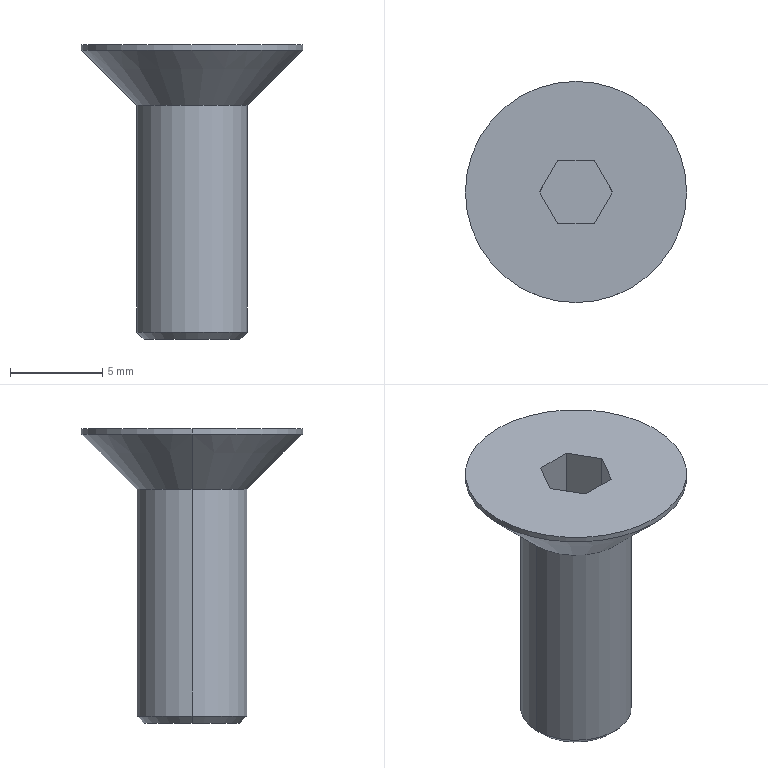Part | Creo | 1 solid | 17 faces | box 12 x 12 x 16 mm | volume 548.89 mm3 | plane 9 | cone 4 | cylinder 4 | commonest cylinder face diameters 6 x2 12 x2
STEP:
#1=CARTESIAN_POINT('',(-332.6,330.,200.));
#2=VERTEX_POINT('',#1);
#3=CARTESIAN_POINT('',(-327.4,330.,200.));
#4=VERTEX_POINT('',#3);
#5=CARTESIAN_POINT('',(-330.,330.,200.));
#6=DIRECTION('',(0.,0.,-1.));
#7=DIRECTION('',(-1.,0.,0.));
#8=AXIS2_PLACEMENT_3D('',#5,#6,#7);
#9=CIRCLE('',#8,2.6);
#10=EDGE_CURVE('',#2,#4,#9,.T.);
#11=ORIENTED_EDGE('',*,*,#10,.F.);
#12=CARTESIAN_POINT('',(-330.,330.,200.));
#13=DIRECTION('',(0.,0.,-1.));
#14=DIRECTION('',(1.,0.,0.));
#15=AXIS2_PLACEMENT_3D('',#12,#13,#14);
#16=CIRCLE('',#15,2.6);
#17=EDGE_CURVE('',#4,#2,#16,.T.);
#18=ORIENTED_EDGE('',*,*,#17,.F.);
#19=EDGE_LOOP('',(#11,#18));
#20=FACE_OUTER_BOUND('',#19,.F.);
#21=CARTESIAN_POINT('',(-326.825,330.,200.));
#22=DIRECTION('',(0.,0.,-1.));
#23=DIRECTION('',(-1.,0.,0.));
#24=AXIS2_PLACEMENT_3D('',#21,#22,#23);
#25=PLANE('',#24);
#26=ADVANCED_FACE('',(#20),#25,.T.);
#27=CARTESIAN_POINT('',(-333.,330.,200.4));
#28=VERTEX_POINT('',#27);
#29=CARTESIAN_POINT('',(-327.,330.,200.4));
#30=VERTEX_POINT('',#29);
#31=CARTESIAN_POINT('',(-330.,330.,200.4));
#32=DIRECTION('',(0.,0.,-1.));
#33=DIRECTION('',(-1.,0.,0.));
#34=AXIS2_PLACEMENT_3D('',#31,#32,#33);
#35=CIRCLE('',#34,3.);
#36=EDGE_CURVE('',#28,#30,#35,.T.);
#37=ORIENTED_EDGE('',*,*,#36,.F.);
#38=CARTESIAN_POINT('',(-332.6,330.,200.));
#39=DIRECTION('',(-0.7071,0.,0.7071));
#40=VECTOR('',#39,0.5657);
#41=LINE('',#38,#40);
#42=EDGE_CURVE('',#2,#28,#41,.T.);
#43=ORIENTED_EDGE('',*,*,#42,.F.);
#44=ORIENTED_EDGE('',*,*,#10,.T.);
#45=CARTESIAN_POINT('',(-327.4,330.,200.));
#46=DIRECTION('',(0.7071,0.,0.7071));
#47=VECTOR('',#46,0.5657);
#48=LINE('',#45,#47);
#49=EDGE_CURVE('',#4,#30,#48,.T.);
#50=ORIENTED_EDGE('',*,*,#49,.T.);
#51=EDGE_LOOP('',(#37,#43,#44,#50));
#52=FACE_OUTER_BOUND('',#51,.F.);
#53=CARTESIAN_POINT('',(-330.,330.,200.2));
#54=DIRECTION('',(0.,0.,1.));
#55=DIRECTION('',(1.,0.,0.));
#56=AXIS2_PLACEMENT_3D('',#53,#54,#55);
#57=CONICAL_SURFACE('',#56,2.8,45.);
#58=ADVANCED_FACE('',(#52),#57,.T.);
#59=ORIENTED_EDGE('',*,*,#36,.T.);
#60=CARTESIAN_POINT('',(-327.,330.,212.7));
#61=VERTEX_POINT('',#60);
#62=CARTESIAN_POINT('',(-327.,330.,200.4));
#63=DIRECTION('',(0.,0.,1.));
#64=VECTOR('',#63,12.3);
#65=LINE('',#62,#64);
#66=EDGE_CURVE('',#30,#61,#65,.T.);
#67=ORIENTED_EDGE('',*,*,#66,.T.);
#68=CARTESIAN_POINT('',(-333.,330.,212.7));
#69=VERTEX_POINT('',#68);
#70=CARTESIAN_POINT('',(-330.,330.,212.7));
#71=DIRECTION('',(0.,0.,1.));
#72=DIRECTION('',(1.,0.,0.));
#73=AXIS2_PLACEMENT_3D('',#70,#71,#72);
#74=CIRCLE('',#73,3.);
#75=EDGE_CURVE('',#61,#69,#74,.T.);
#76=ORIENTED_EDGE('',*,*,#75,.T.);
#77=CARTESIAN_POINT('',(-333.,330.,200.4));
#78=DIRECTION('',(0.,0.,1.));
#79=VECTOR('',#78,12.3);
#80=LINE('',#77,#79);
#81=EDGE_CURVE('',#28,#69,#80,.T.);
#82=ORIENTED_EDGE('',*,*,#81,.F.);
#83=EDGE_LOOP('',(#59,#67,#76,#82));
#84=FACE_OUTER_BOUND('',#83,.F.);
#85=CARTESIAN_POINT('',(-330.,330.,216.307));
#86=DIRECTION('',(0.,0.,1.));
#87=DIRECTION('',(1.,0.,0.));
#88=AXIS2_PLACEMENT_3D('',#85,#86,#87);
#89=CYLINDRICAL_SURFACE('',#88,3.);
#90=ADVANCED_FACE('',(#84),#89,.T.);
#91=CARTESIAN_POINT('',(-330.,330.,200.4));
#92=DIRECTION('',(0.,0.,-1.));
#93=DIRECTION('',(1.,0.,0.));
#94=AXIS2_PLACEMENT_3D('',#91,#92,#93);
#95=CIRCLE('',#94,3.);
#96=EDGE_CURVE('',#30,#28,#95,.T.);
#97=ORIENTED_EDGE('',*,*,#96,.T.);
#98=ORIENTED_EDGE('',*,*,#81,.T.);
#99=CARTESIAN_POINT('',(-330.,330.,212.7));
#100=DIRECTION('',(0.,0.,1.));
#101=DIRECTION('',(-1.,0.,0.));
#102=AXIS2_PLACEMENT_3D('',#99,#100,#101);
#103=CIRCLE('',#102,3.);
#104=EDGE_CURVE('',#69,#61,#103,.T.);
#105=ORIENTED_EDGE('',*,*,#104,.T.);
#106=ORIENTED_EDGE('',*,*,#66,.F.);
#107=EDGE_LOOP('',(#97,#98,#105,#106));
#108=FACE_OUTER_BOUND('',#107,.F.);
#109=CARTESIAN_POINT('',(-330.,330.,216.307));
#110=DIRECTION('',(0.,0.,1.));
#111=DIRECTION('',(1.,0.,0.));
#112=AXIS2_PLACEMENT_3D('',#109,#110,#111);
#113=CYLINDRICAL_SURFACE('',#112,3.);
#114=ADVANCED_FACE('',(#108),#113,.T.);
#115=ORIENTED_EDGE('',*,*,#96,.F.);
#116=ORIENTED_EDGE('',*,*,#49,.F.);
#117=ORIENTED_EDGE('',*,*,#17,.T.);
#118=ORIENTED_EDGE('',*,*,#42,.T.);
#119=EDGE_LOOP('',(#115,#116,#117,#118));
#120=FACE_OUTER_BOUND('',#119,.F.);
#121=CARTESIAN_POINT('',(-330.,330.,200.2));
#122=DIRECTION('',(0.,0.,1.));
#123=DIRECTION('',(1.,0.,0.));
#124=AXIS2_PLACEMENT_3D('',#121,#122,#123);
#125=CONICAL_SURFACE('',#124,2.8,45.);
#126=ADVANCED_FACE('',(#120),#125,.T.);
#127=ORIENTED_EDGE('',*,*,#104,.F.);
#128=CARTESIAN_POINT('',(-336.,330.,215.7));
#129=VERTEX_POINT('',#128);
#130=CARTESIAN_POINT('',(-333.,330.,212.7));
#131=DIRECTION('',(-0.7071,0.,0.7071));
#132=VECTOR('',#131,4.243);
#133=LINE('',#130,#132);
#134=EDGE_CURVE('',#69,#129,#133,.T.);
#135=ORIENTED_EDGE('',*,*,#134,.T.);
#136=CARTESIAN_POINT('',(-324.,330.,215.7));
#137=VERTEX_POINT('',#136);
#138=CARTESIAN_POINT('',(-330.,330.,215.7));
#139=DIRECTION('',(0.,0.,-1.));
#140=DIRECTION('',(1.,0.,0.));
#141=AXIS2_PLACEMENT_3D('',#138,#139,#140);
#142=CIRCLE('',#141,6.);
#143=EDGE_CURVE('',#137,#129,#142,.T.);
#144=ORIENTED_EDGE('',*,*,#143,.F.);
#145=CARTESIAN_POINT('',(-327.,330.,212.7));
#146=DIRECTION('',(0.7071,0.,0.7071));
#147=VECTOR('',#146,4.243);
#148=LINE('',#145,#147);
#149=EDGE_CURVE('',#61,#137,#148,.T.);
#150=ORIENTED_EDGE('',*,*,#149,.F.);
#151=EDGE_LOOP('',(#127,#135,#144,#150));
#152=FACE_OUTER_BOUND('',#151,.F.);
#153=CARTESIAN_POINT('',(-330.,330.,214.2));
#154=DIRECTION('',(0.,0.,1.));
#155=DIRECTION('',(1.,0.,0.));
#156=AXIS2_PLACEMENT_3D('',#153,#154,#155);
#157=CONICAL_SURFACE('',#156,4.5,45.);
#158=ADVANCED_FACE('',(#152),#157,.T.);
#159=ORIENTED_EDGE('',*,*,#75,.F.);
#160=ORIENTED_EDGE('',*,*,#149,.T.);
#161=CARTESIAN_POINT('',(-330.,330.,215.7));
#162=DIRECTION('',(0.,0.,-1.));
#163=DIRECTION('',(-1.,0.,0.));
#164=AXIS2_PLACEMENT_3D('',#161,#162,#163);
#165=CIRCLE('',#164,6.);
#166=EDGE_CURVE('',#129,#137,#165,.T.);
#167=ORIENTED_EDGE('',*,*,#166,.F.);
#168=ORIENTED_EDGE('',*,*,#134,.F.);
#169=EDGE_LOOP('',(#159,#160,#167,#168));
#170=FACE_OUTER_BOUND('',#169,.F.);
#171=CARTESIAN_POINT('',(-330.,330.,214.2));
#172=DIRECTION('',(0.,0.,1.));
#173=DIRECTION('',(1.,0.,0.));
#174=AXIS2_PLACEMENT_3D('',#171,#172,#173);
#175=CONICAL_SURFACE('',#174,4.5,45.);
#176=ADVANCED_FACE('',(#170),#175,.T.);
#177=ORIENTED_EDGE('',*,*,#166,.T.);
#178=CARTESIAN_POINT('',(-324.,330.,216.));
#179=VERTEX_POINT('',#178);
#180=CARTESIAN_POINT('',(-324.,330.,215.7));
#181=DIRECTION('',(0.,0.,1.));
#182=VECTOR('',#181,0.3);
#183=LINE('',#180,#182);
#184=EDGE_CURVE('',#137,#179,#183,.T.);
#185=ORIENTED_EDGE('',*,*,#184,.T.);
#186=CARTESIAN_POINT('',(-336.,330.,216.));
#187=VERTEX_POINT('',#186);
#188=CARTESIAN_POINT('',(-330.,330.,216.));
#189=DIRECTION('',(0.,0.,1.));
#190=DIRECTION('',(1.,0.,0.));
#191=AXIS2_PLACEMENT_3D('',#188,#189,#190);
#192=CIRCLE('',#191,6.);
#193=EDGE_CURVE('',#179,#187,#192,.T.);
#194=ORIENTED_EDGE('',*,*,#193,.T.);
#195=CARTESIAN_POINT('',(-336.,330.,215.7));
#196=DIRECTION('',(0.,0.,1.));
#197=VECTOR('',#196,0.3);
#198=LINE('',#195,#197);
#199=EDGE_CURVE('',#129,#187,#198,.T.);
#200=ORIENTED_EDGE('',*,*,#199,.F.);
#201=EDGE_LOOP('',(#177,#185,#194,#200));
#202=FACE_OUTER_BOUND('',#201,.F.);
#203=CARTESIAN_POINT('',(-330.,330.,216.397));
#204=DIRECTION('',(0.,0.,1.));
#205=DIRECTION('',(1.,0.,0.));
#206=AXIS2_PLACEMENT_3D('',#203,#204,#205);
#207=CYLINDRICAL_SURFACE('',#206,6.);
#208=ADVANCED_FACE('',(#202),#207,.T.);
#209=ORIENTED_EDGE('',*,*,#143,.T.);
#210=ORIENTED_EDGE('',*,*,#199,.T.);
#211=CARTESIAN_POINT('',(-330.,330.,216.));
#212=DIRECTION('',(0.,0.,1.));
#213=DIRECTION('',(-1.,0.,0.));
#214=AXIS2_PLACEMENT_3D('',#211,#212,#213);
#215=CIRCLE('',#214,6.);
#216=EDGE_CURVE('',#187,#179,#215,.T.);
#217=ORIENTED_EDGE('',*,*,#216,.T.);
#218=ORIENTED_EDGE('',*,*,#184,.F.);
#219=EDGE_LOOP('',(#209,#210,#217,#218));
#220=FACE_OUTER_BOUND('',#219,.F.);
#221=CARTESIAN_POINT('',(-330.,330.,216.397));
#222=DIRECTION('',(0.,0.,1.));
#223=DIRECTION('',(1.,0.,0.));
#224=AXIS2_PLACEMENT_3D('',#221,#222,#223);
#225=CYLINDRICAL_SURFACE('',#224,6.);
#226=ADVANCED_FACE('',(#220),#225,.T.);
#227=ORIENTED_EDGE('',*,*,#193,.F.);
#228=ORIENTED_EDGE('',*,*,#216,.F.);
#229=EDGE_LOOP('',(#227,#228));
#230=FACE_OUTER_BOUND('',#229,.F.);
#231=CARTESIAN_POINT('',(-330.992,331.719,216.));
#232=VERTEX_POINT('',#231);
#233=CARTESIAN_POINT('',(-329.008,331.719,216.));
#234=VERTEX_POINT('',#233);
#235=CARTESIAN_POINT('',(-330.992,331.719,216.));
#236=DIRECTION('',(1.,0.,0.));
#237=VECTOR('',#236,1.984);
#238=LINE('',#235,#237);
#239=EDGE_CURVE('',#232,#234,#238,.T.);
#240=ORIENTED_EDGE('',*,*,#239,.F.);
#241=CARTESIAN_POINT('',(-331.984,330.,216.));
#242=VERTEX_POINT('',#241);
#243=CARTESIAN_POINT('',(-331.984,330.,216.));
#244=DIRECTION('',(0.5,0.866,0.));
#245=VECTOR('',#244,1.984);
#246=LINE('',#243,#245);
#247=EDGE_CURVE('',#242,#232,#246,.T.);
#248=ORIENTED_EDGE('',*,*,#247,.F.);
#249=CARTESIAN_POINT('',(-330.992,328.281,216.));
#250=VERTEX_POINT('',#249);
#251=CARTESIAN_POINT('',(-330.992,328.281,216.));
#252=DIRECTION('',(-0.5,0.866,0.));
#253=VECTOR('',#252,1.984);
#254=LINE('',#251,#253);
#255=EDGE_CURVE('',#250,#242,#254,.T.);
#256=ORIENTED_EDGE('',*,*,#255,.F.);
#257=CARTESIAN_POINT('',(-329.008,328.281,216.));
#258=VERTEX_POINT('',#257);
#259=CARTESIAN_POINT('',(-329.008,328.281,216.));
#260=DIRECTION('',(-1.,0.,0.));
#261=VECTOR('',#260,1.984);
#262=LINE('',#259,#261);
#263=EDGE_CURVE('',#258,#250,#262,.T.);
#264=ORIENTED_EDGE('',*,*,#263,.F.);
#265=CARTESIAN_POINT('',(-328.016,330.,216.));
#266=VERTEX_POINT('',#265);
#267=CARTESIAN_POINT('',(-328.016,330.,216.));
#268=DIRECTION('',(-0.5,-0.866,0.));
#269=VECTOR('',#268,1.984);
#270=LINE('',#267,#269);
#271=EDGE_CURVE('',#266,#258,#270,.T.);
#272=ORIENTED_EDGE('',*,*,#271,.F.);
#273=CARTESIAN_POINT('',(-329.008,331.719,216.));
#274=DIRECTION('',(0.5,-0.866,0.));
#275=VECTOR('',#274,1.984);
#276=LINE('',#273,#275);
#277=EDGE_CURVE('',#234,#266,#276,.T.);
#278=ORIENTED_EDGE('',*,*,#277,.F.);
#279=EDGE_LOOP('',(#240,#248,#256,#264,#272,#278));
#280=FACE_BOUND('',#279,.F.);
#281=CARTESIAN_POINT('',(-330.,330.,216.));
#282=DIRECTION('',(0.,0.,1.));
#283=DIRECTION('',(1.,0.,0.));
#284=AXIS2_PLACEMENT_3D('',#281,#282,#283);
#285=PLANE('',#284);
#286=ADVANCED_FACE('',(#230,#280),#285,.T.);
#287=ORIENTED_EDGE('',*,*,#239,.T.);
#288=CARTESIAN_POINT('',(-329.008,331.719,212.031));
#289=VERTEX_POINT('',#288);
#290=CARTESIAN_POINT('',(-329.008,331.719,216.));
#291=DIRECTION('',(0.,0.,-1.));
#292=VECTOR('',#291,3.969);
#293=LINE('',#290,#292);
#294=EDGE_CURVE('',#234,#289,#293,.T.);
#295=ORIENTED_EDGE('',*,*,#294,.T.);
#296=CARTESIAN_POINT('',(-330.992,331.719,212.031));
#297=VERTEX_POINT('',#296);
#298=CARTESIAN_POINT('',(-330.992,331.719,212.031));
#299=DIRECTION('',(1.,0.,0.));
#300=VECTOR('',#299,1.984);
#301=LINE('',#298,#300);
#302=EDGE_CURVE('',#297,#289,#301,.T.);
#303=ORIENTED_EDGE('',*,*,#302,.F.);
#304=CARTESIAN_POINT('',(-330.992,331.719,216.));
#305=DIRECTION('',(0.,0.,-1.));
#306=VECTOR('',#305,3.969);
#307=LINE('',#304,#306);
#308=EDGE_CURVE('',#232,#297,#307,.T.);
#309=ORIENTED_EDGE('',*,*,#308,.F.);
#310=EDGE_LOOP('',(#287,#295,#303,#309));
#311=FACE_OUTER_BOUND('',#310,.F.);
#312=CARTESIAN_POINT('',(-329.008,331.719,211.942));
#313=DIRECTION('',(0.,1.,0.));
#314=DIRECTION('',(-1.,0.,0.));
#315=AXIS2_PLACEMENT_3D('',#312,#313,#314);
#316=PLANE('',#315);
#317=ADVANCED_FACE('',(#311),#316,.F.);
#318=ORIENTED_EDGE('',*,*,#277,.T.);
#319=CARTESIAN_POINT('',(-328.016,330.,212.031));
#320=VERTEX_POINT('',#319);
#321=CARTESIAN_POINT('',(-328.016,330.,216.));
#322=DIRECTION('',(0.,0.,-1.));
#323=VECTOR('',#322,3.969);
#324=LINE('',#321,#323);
#325=EDGE_CURVE('',#266,#320,#324,.T.);
#326=ORIENTED_EDGE('',*,*,#325,.T.);
#327=CARTESIAN_POINT('',(-328.016,330.,212.031));
#328=DIRECTION('',(-0.5,0.866,0.));
#329=VECTOR('',#328,1.984);
#330=LINE('',#327,#329);
#331=EDGE_CURVE('',#320,#289,#330,.T.);
#332=ORIENTED_EDGE('',*,*,#331,.T.);
#333=ORIENTED_EDGE('',*,*,#294,.F.);
#334=EDGE_LOOP('',(#318,#326,#332,#333));
#335=FACE_OUTER_BOUND('',#334,.F.);
#336=CARTESIAN_POINT('',(-328.016,330.,211.942));
#337=DIRECTION('',(0.866,0.5,0.));
#338=DIRECTION('',(-0.5,0.866,0.));
#339=AXIS2_PLACEMENT_3D('',#336,#337,#338);
#340=PLANE('',#339);
#341=ADVANCED_FACE('',(#335),#340,.F.);
#342=ORIENTED_EDGE('',*,*,#271,.T.);
#343=CARTESIAN_POINT('',(-329.008,328.281,212.031));
#344=VERTEX_POINT('',#343);
#345=CARTESIAN_POINT('',(-329.008,328.281,216.));
#346=DIRECTION('',(0.,0.,-1.));
#347=VECTOR('',#346,3.969);
#348=LINE('',#345,#347);
#349=EDGE_CURVE('',#258,#344,#348,.T.);
#350=ORIENTED_EDGE('',*,*,#349,.T.);
#351=CARTESIAN_POINT('',(-329.008,328.281,212.031));
#352=DIRECTION('',(0.5,0.866,0.));
#353=VECTOR('',#352,1.984);
#354=LINE('',#351,#353);
#355=EDGE_CURVE('',#344,#320,#354,.T.);
#356=ORIENTED_EDGE('',*,*,#355,.T.);
#357=ORIENTED_EDGE('',*,*,#325,.F.);
#358=EDGE_LOOP('',(#342,#350,#356,#357));
#359=FACE_OUTER_BOUND('',#358,.F.);
#360=CARTESIAN_POINT('',(-329.008,328.281,211.942));
#361=DIRECTION('',(0.866,-0.5,0.));
#362=DIRECTION('',(0.5,0.866,0.));
#363=AXIS2_PLACEMENT_3D('',#360,#361,#362);
#364=PLANE('',#363);
#365=ADVANCED_FACE('',(#359),#364,.F.);
#366=ORIENTED_EDGE('',*,*,#263,.T.);
#367=CARTESIAN_POINT('',(-330.992,328.281,212.031));
#368=VERTEX_POINT('',#367);
#369=CARTESIAN_POINT('',(-330.992,328.281,216.));
#370=DIRECTION('',(0.,0.,-1.));
#371=VECTOR('',#370,3.969);
#372=LINE('',#369,#371);
#373=EDGE_CURVE('',#250,#368,#372,.T.);
#374=ORIENTED_EDGE('',*,*,#373,.T.);
#375=CARTESIAN_POINT('',(-329.008,328.281,212.031));
#376=DIRECTION('',(-1.,0.,0.));
#377=VECTOR('',#376,1.984);
#378=LINE('',#375,#377);
#379=EDGE_CURVE('',#344,#368,#378,.T.);
#380=ORIENTED_EDGE('',*,*,#379,.F.);
#381=ORIENTED_EDGE('',*,*,#349,.F.);
#382=EDGE_LOOP('',(#366,#374,#380,#381));
#383=FACE_OUTER_BOUND('',#382,.F.);
#384=CARTESIAN_POINT('',(-330.992,328.281,211.942));
#385=DIRECTION('',(0.,-1.,0.));
#386=DIRECTION('',(1.,0.,0.));
#387=AXIS2_PLACEMENT_3D('',#384,#385,#386);
#388=PLANE('',#387);
#389=ADVANCED_FACE('',(#383),#388,.F.);
#390=ORIENTED_EDGE('',*,*,#255,.T.);
#391=CARTESIAN_POINT('',(-331.984,330.,212.031));
#392=VERTEX_POINT('',#391);
#393=CARTESIAN_POINT('',(-331.984,330.,216.));
#394=DIRECTION('',(0.,0.,-1.));
#395=VECTOR('',#394,3.969);
#396=LINE('',#393,#395);
#397=EDGE_CURVE('',#242,#392,#396,.T.);
#398=ORIENTED_EDGE('',*,*,#397,.T.);
#399=CARTESIAN_POINT('',(-331.984,330.,212.031));
#400=DIRECTION('',(0.5,-0.866,0.));
#401=VECTOR('',#400,1.984);
#402=LINE('',#399,#401);
#403=EDGE_CURVE('',#392,#368,#402,.T.);
#404=ORIENTED_EDGE('',*,*,#403,.T.);
#405=ORIENTED_EDGE('',*,*,#373,.F.);
#406=EDGE_LOOP('',(#390,#398,#404,#405));
#407=FACE_OUTER_BOUND('',#406,.F.);
#408=CARTESIAN_POINT('',(-331.984,330.,211.942));
#409=DIRECTION('',(-0.866,-0.5,0.));
#410=DIRECTION('',(0.5,-0.866,0.));
#411=AXIS2_PLACEMENT_3D('',#408,#409,#410);
#412=PLANE('',#411);
#413=ADVANCED_FACE('',(#407),#412,.F.);
#414=ORIENTED_EDGE('',*,*,#247,.T.);
#415=ORIENTED_EDGE('',*,*,#308,.T.);
#416=CARTESIAN_POINT('',(-330.992,331.719,212.031));
#417=DIRECTION('',(-0.5,-0.866,0.));
#418=VECTOR('',#417,1.984);
#419=LINE('',#416,#418);
#420=EDGE_CURVE('',#297,#392,#419,.T.);
#421=ORIENTED_EDGE('',*,*,#420,.T.);
#422=ORIENTED_EDGE('',*,*,#397,.F.);
#423=EDGE_LOOP('',(#414,#415,#421,#422));
#424=FACE_OUTER_BOUND('',#423,.F.);
#425=CARTESIAN_POINT('',(-330.992,331.719,211.942));
#426=DIRECTION('',(-0.866,0.5,0.));
#427=DIRECTION('',(-0.5,-0.866,0.));
#428=AXIS2_PLACEMENT_3D('',#425,#426,#427);
#429=PLANE('',#428);
#430=ADVANCED_FACE('',(#424),#429,.F.);
#431=ORIENTED_EDGE('',*,*,#302,.T.);
#432=ORIENTED_EDGE('',*,*,#331,.F.);
#433=ORIENTED_EDGE('',*,*,#355,.F.);
#434=ORIENTED_EDGE('',*,*,#379,.T.);
#435=ORIENTED_EDGE('',*,*,#403,.F.);
#436=ORIENTED_EDGE('',*,*,#420,.F.);
#437=EDGE_LOOP('',(#431,#432,#433,#434,#435,#436));
#438=FACE_OUTER_BOUND('',#437,.F.);
#439=CARTESIAN_POINT('',(-330.992,331.719,212.031));
#440=DIRECTION('',(0.,0.,1.));
#441=DIRECTION('',(1.,0.,0.));
#442=AXIS2_PLACEMENT_3D('',#439,#440,#441);
#443=PLANE('',#442);
#444=ADVANCED_FACE('',(#438),#443,.T.);
#445=CLOSED_SHELL('',(#26,#58,#90,#114,#126,#158,#176,#208,#226,#286,#317,#341,#365,#389,#413,#430,#444));
#446=MANIFOLD_SOLID_BREP('',#445);
#447=(LENGTH_UNIT()NAMED_UNIT(*)SI_UNIT(.MILLI.,.METRE.));
#448=UNCERTAINTY_MEASURE_WITH_UNIT(LENGTH_MEASURE(0.002332),#447,'','');
#449=(NAMED_UNIT(*)PLANE_ANGLE_UNIT()SI_UNIT($,.RADIAN.));
#450=PLANE_ANGLE_MEASURE_WITH_UNIT(PLANE_ANGLE_MEASURE(0.01745),#449);
#451=(CONVERSION_BASED_UNIT('DEGREE',#450)NAMED_UNIT(*)PLANE_ANGLE_UNIT());
#452=(NAMED_UNIT(*)SI_UNIT($,.STERADIAN.)SOLID_ANGLE_UNIT());
#453=(GEOMETRIC_REPRESENTATION_CONTEXT(3)GLOBAL_UNCERTAINTY_ASSIGNED_CONTEXT((#448))GLOBAL_UNIT_ASSIGNED_CONTEXT((#447,#451,#452))REPRESENTATION_CONTEXT('',''));
#454=ADVANCED_BREP_SHAPE_REPRESENTATION('',(#446),#453);